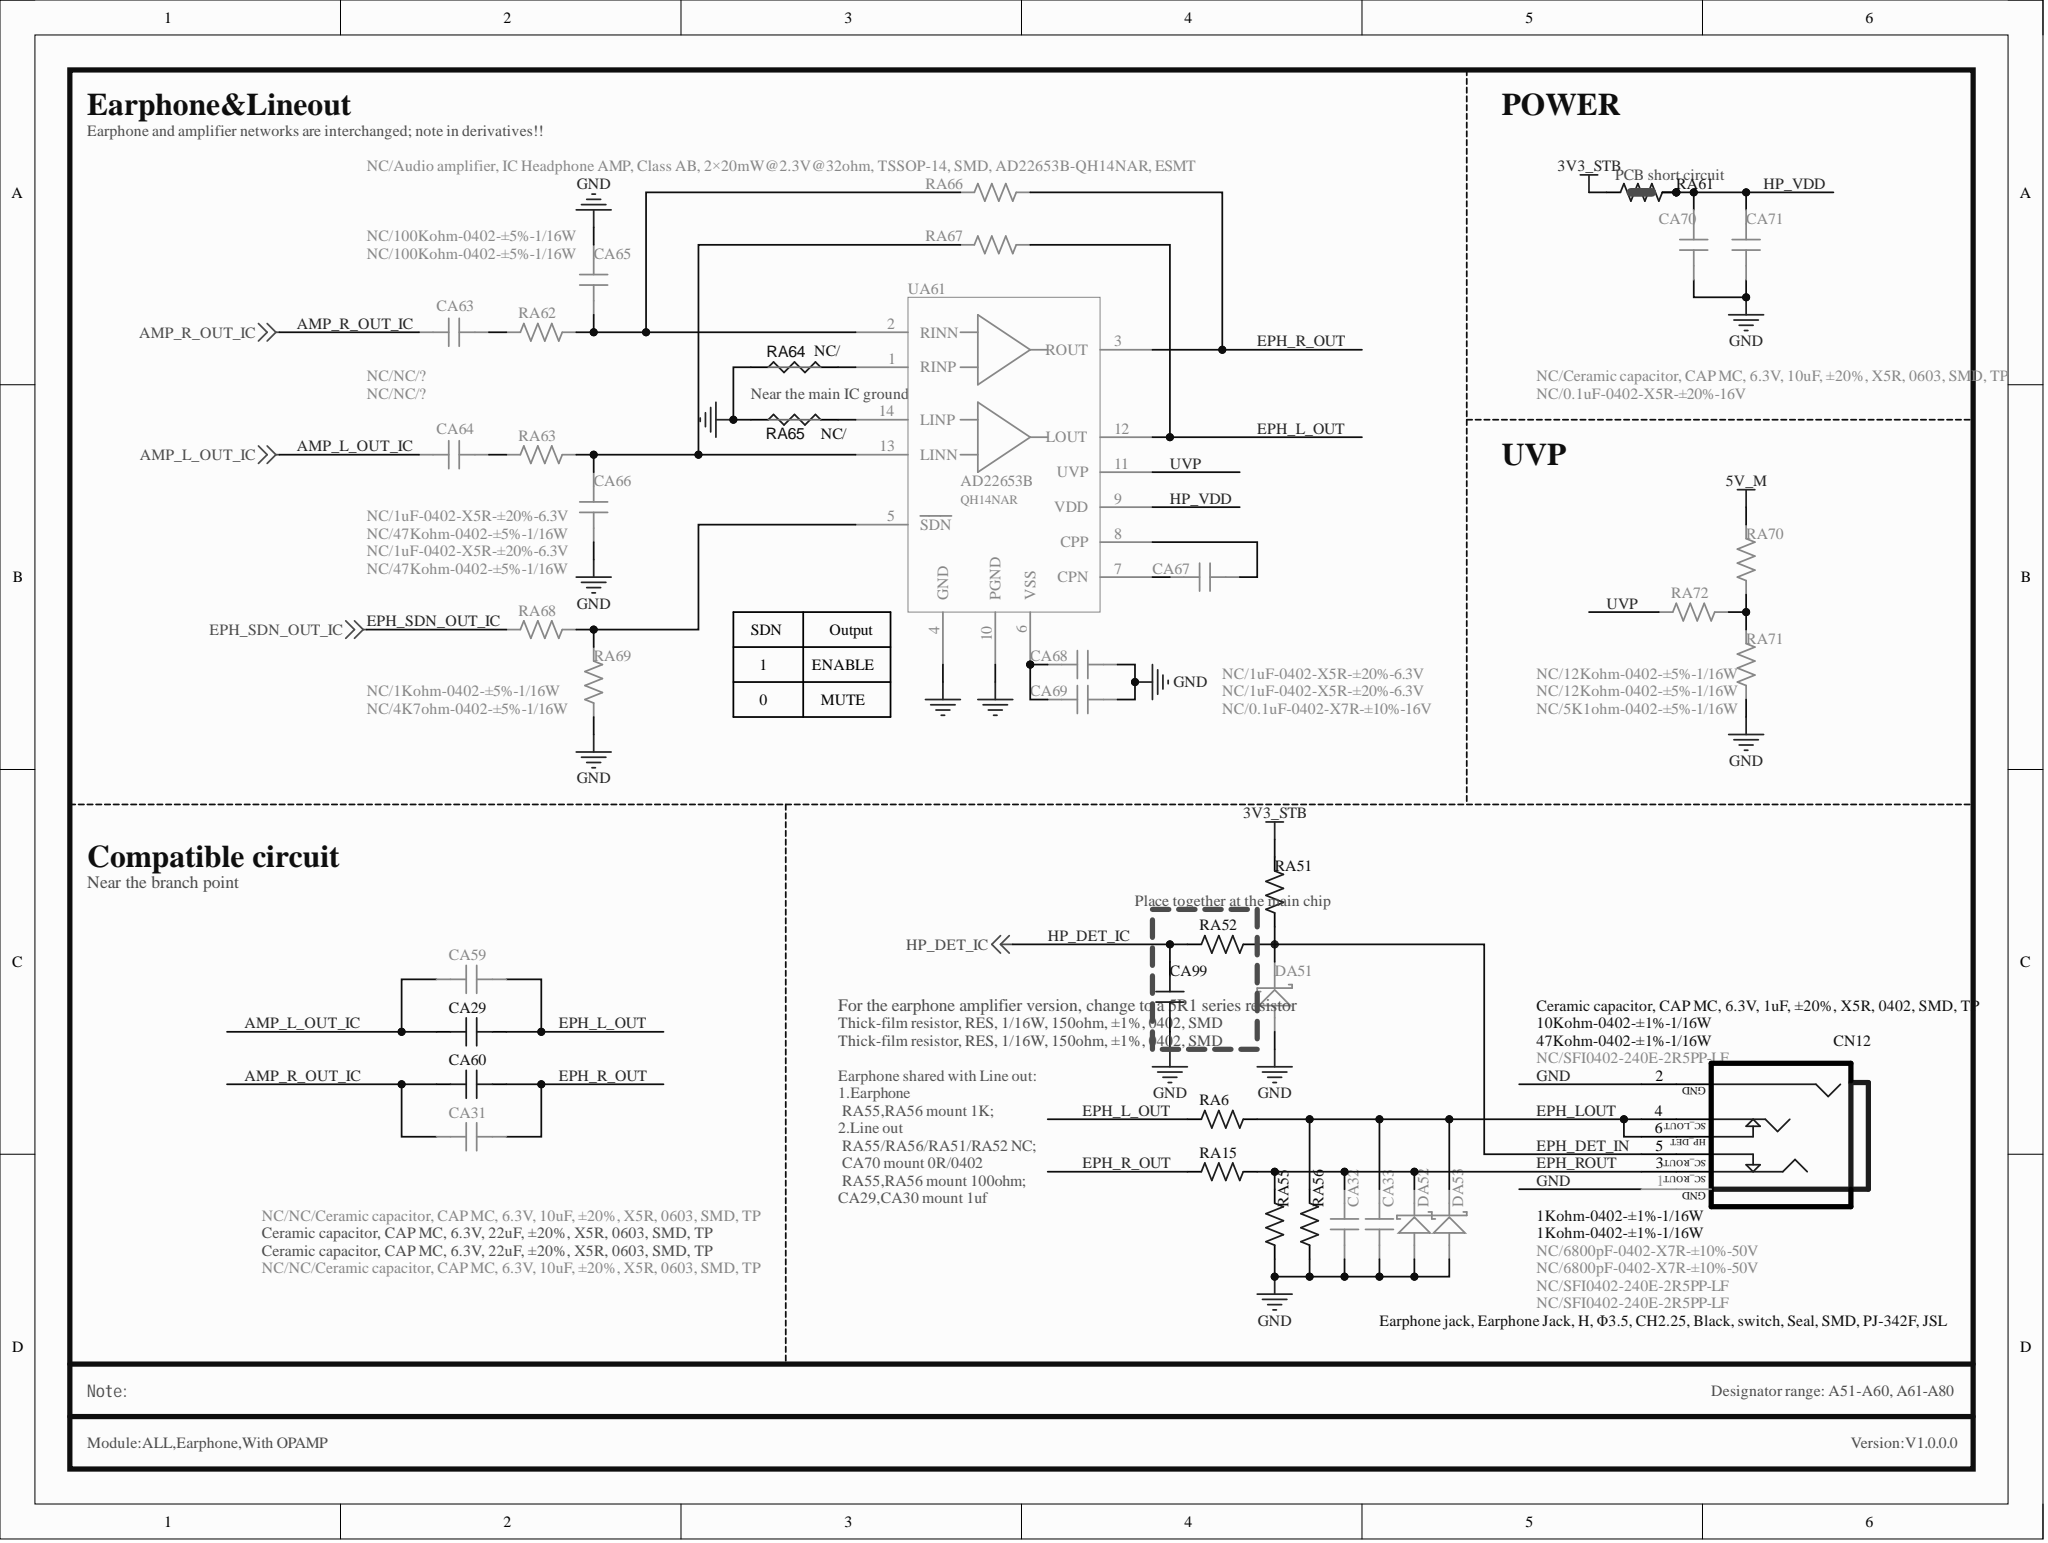Circuit board | Altium Designer | 541 parts | 263 nets | one sheet of the schematic
Parts on this sheet (reference | value | footprint):
CA29 | Ceramic capacitor, CAP MC, 6.3V, 22uF, ±20%, X5R, 0603, SMD, TP | C0603
CA31 | NC/NC/Ceramic capacitor, CAP MC, 6.3V, 10uF, ±20%, X5R, 0603, SMD, TP | C0603
CA32 | NC/6800pF-0402-X7R-±10%-50V | C0402
CA33 | NC/6800pF-0402-X7R-±10%-50V | C0402
CA59 | NC/NC/Ceramic capacitor, CAP MC, 6.3V, 10uF, ±20%, X5R, 0603, SMD, TP | C0603
CA60 | Ceramic capacitor, CAP MC, 6.3V, 22uF, ±20%, X5R, 0603, SMD, TP | C0603
CA63 | NC/1uF-0402-X5R-±20%-6.3V | C0402
CA64 | NC/1uF-0402-X5R-±20%-6.3V | C0402
CA65 | NC/NC/? | C0402
CA66 | NC/NC/? | C0402
CA67 | NC/1uF-0402-X5R-±20%-6.3V | C0402
CA68 | NC/1uF-0402-X5R-±20%-6.3V | C0402
CA69 | NC/0.1uF-0402-X7R-±10%-16V | C0402
CA70 | NC/Ceramic capacitor, CAP MC, 6.3V, 10uF, ±20%, X5R, 0603, SMD, TP | C0603
CA71 | NC/0.1uF-0402-X5R-±20%-16V | C0402
CA99 | Ceramic capacitor, CAP MC, 6.3V, 1uF, ±20%, X5R, 0402, SMD, TP | C0402
CN12 | Earphone jack, Earphone Jack, H, F3.5, CH2.25, Black, switch, Seal, SMD, PJ-342F, JSL | PHONE-HS-29
DA51 | NC/SFI0402-240E-2R5PP-LF | DIODE-S0402
DA52 | NC/SFI0402-240E-2R5PP-LF | DIODE-S0402
DA53 | NC/SFI0402-240E-2R5PP-LF | DIODE-S0402
RA6 | Thick-film resistor, RES, 1/16W, 150ohm, ±1%, 0402, SMD | R0402
RA15 | Thick-film resistor, RES, 1/16W, 150ohm, ±1%, 0402, SMD | R0402
RA51 | 47Kohm-0402-±1%-1/16W | R0402
RA52 | 10Kohm-0402-±1%-1/16W | R0402
RA55 | 1Kohm-0402-±1%-1/16W | R0402
RA56 | 1Kohm-0402-±1%-1/16W | R0402
RA61 | NC/NC/0ohm-0402-PCB | R0402SC
RA62 | NC/47Kohm-0402-±5%-1/16W | R0402
RA63 | NC/47Kohm-0402-±5%-1/16W | R0402
RA64 | NC/ | GND
RA65 | NC/ | GND
RA66 | NC/100Kohm-0402-±5%-1/16W | R0402
RA67 | NC/100Kohm-0402-±5%-1/16W | R0402
RA68 | NC/1Kohm-0402-±5%-1/16W | R0402
RA69 | NC/4K7ohm-0402-±5%-1/16W | R0402
RA70 | NC/12Kohm-0402-±5%-1/16W | R0402
RA71 | NC/5K1ohm-0402-±5%-1/16W | R0402
RA72 | NC/12Kohm-0402-±5%-1/16W | R0402
UA61 | NC/Audio amplifier, IC Headphone AMP, Class AB, 2×20mW@2.3V@32ohm, TSSOP-14, SMD, AD22653B-QH14NAR, ESMT | SSOP14/0.65-1
Nets of these parts (net: part-pin ...):
UVP: RA72-2 UA61-11
NetRA70_1: RA70-1 RA71-2 RA72-1
NetRA68_2: RA68-2 RA69-2 UA61-5
NetRA65_JP_1K: RA65-JP_1K UA61-14
NetRA64_JP_1K: RA64-JP_1K UA61-1
NetCA68_1: CA68-1 CA69-1 UA61-6
NetCA67_2: CA67-2 UA61-7
NetCA67_1: CA67-1 UA61-8
NetCA66_2: CA66-2 RA63-2 RA67-1 UA61-13
NetCA65_1: CA65-1 RA62-2 RA66-1 UA61-2
NetCA64_2: CA64-2 RA63-1
NetCA63_2: CA63-2 RA62-1
HP_VDD: CA70-1 CA71-1 RA61-2 RA61-3 UA61-9
HP_DET_IC: CA99-2 RA52-2
GND: CA32-2 CA33-2 CA65-2 CA66-1 CA68-2 CA69-2 CA70-2 CA71-2 CA99-1 CN12-1 CN12-2 DA51-A DA52-A DA53-A RA55-1 RA56-1 RA64-JP_2K RA65-JP_2K RA69-1 RA71-1 UA61-4 UA61-10
EPH_SDN_OUT_IC: RA68-1
EPH_ROUT: CA32-1 CN12-3 DA52-K RA15-2 RA55-2
EPH_R_OUT: CA31-2 CA60-2 RA15-1 RA66-2 UA61-3
EPH_LOUT: CA33-1 CN12-4 CN12-6 DA53-K RA6-2 RA56-2
EPH_L_OUT: CA29-2 CA59-2 RA6-1 RA67-2 UA61-12
EPH_DET_IN: CN12-5 DA51-K RA51-1 RA52-1
AMP_R_OUT_IC: CA31-1 CA60-1 CA63-1
AMP_L_OUT_IC: CA29-1 CA59-1 CA64-1
5V_M: RA70-2
3V3_STB: RA51-2 RA61-1